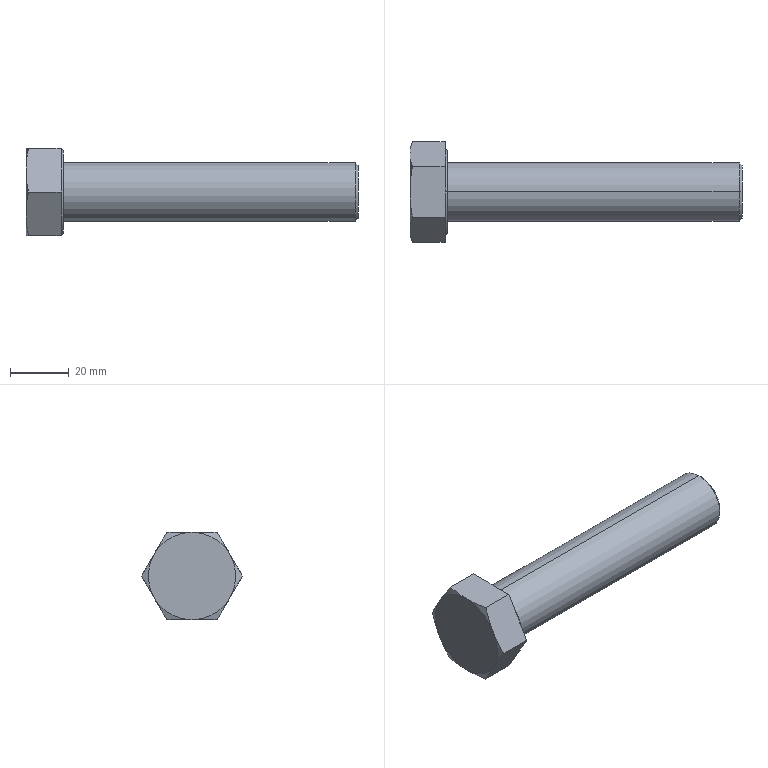Part | 1 solid | 27 faces | box 112.715 x 34.26 x 29.67 mm | volume 40979 mm3 | plane 15 | cone 10 | cylinder 2 | commonest cylinder face diameters 20 x2
STEP:
#1=CARTESIAN_POINT('',(112.715,0.,-9.));
#2=VERTEX_POINT('',#1);
#3=CARTESIAN_POINT('',(112.715,0.,9.));
#4=VERTEX_POINT('',#3);
#5=CARTESIAN_POINT('',(112.715,0.,0.));
#6=DIRECTION('',(1.,0.,0.));
#7=DIRECTION('',(0.,0.,-1.));
#8=AXIS2_PLACEMENT_3D('',#5,#6,#7);
#9=CIRCLE('',#8,9.);
#10=EDGE_CURVE('',#2,#4,#9,.T.);
#11=ORIENTED_EDGE('',*,*,#10,.F.);
#12=CARTESIAN_POINT('',(111.715,0.,-10.));
#13=VERTEX_POINT('',#12);
#14=CARTESIAN_POINT('',(112.715,0.,-9.));
#15=DIRECTION('',(-0.7071,0.,-0.7071));
#16=VECTOR('',#15,1000.);
#17=LINE('',#14,#16);
#18=EDGE_CURVE('',#2,#13,#17,.T.);
#19=ORIENTED_EDGE('',*,*,#18,.T.);
#20=CARTESIAN_POINT('',(111.715,0.,10.));
#21=VERTEX_POINT('',#20);
#22=CARTESIAN_POINT('',(111.715,0.,0.));
#23=DIRECTION('',(-1.,0.,0.));
#24=DIRECTION('',(0.,0.,-1.));
#25=AXIS2_PLACEMENT_3D('',#22,#23,#24);
#26=CIRCLE('',#25,10.);
#27=EDGE_CURVE('',#21,#13,#26,.T.);
#28=ORIENTED_EDGE('',*,*,#27,.F.);
#29=CARTESIAN_POINT('',(112.715,0.,9.));
#30=DIRECTION('',(-0.7071,0.,0.7071));
#31=VECTOR('',#30,1000.);
#32=LINE('',#29,#31);
#33=EDGE_CURVE('',#4,#21,#32,.T.);
#34=ORIENTED_EDGE('',*,*,#33,.F.);
#35=EDGE_LOOP('',(#11,#19,#28,#34));
#36=FACE_OUTER_BOUND('',#35,.T.);
#37=CARTESIAN_POINT('',(112.715,0.,0.));
#38=DIRECTION('',(-1.,0.,0.));
#39=DIRECTION('',(0.,0.,1.));
#40=AXIS2_PLACEMENT_3D('',#37,#38,#39);
#41=CONICAL_SURFACE('',#40,9.,0.7854);
#42=ADVANCED_FACE('',(#36),#41,.T.);
#43=ORIENTED_EDGE('',*,*,#27,.T.);
#44=CARTESIAN_POINT('',(12.715,0.,-10.));
#45=VERTEX_POINT('',#44);
#46=CARTESIAN_POINT('',(112.715,0.,-10.));
#47=DIRECTION('',(-1.,0.,0.));
#48=VECTOR('',#47,1000.);
#49=LINE('',#46,#48);
#50=EDGE_CURVE('',#13,#45,#49,.T.);
#51=ORIENTED_EDGE('',*,*,#50,.T.);
#52=CARTESIAN_POINT('',(12.715,0.,10.));
#53=VERTEX_POINT('',#52);
#54=CARTESIAN_POINT('',(12.715,0.,0.));
#55=DIRECTION('',(1.,0.,0.));
#56=DIRECTION('',(0.,0.,-1.));
#57=AXIS2_PLACEMENT_3D('',#54,#55,#56);
#58=CIRCLE('',#57,10.);
#59=EDGE_CURVE('',#45,#53,#58,.T.);
#60=ORIENTED_EDGE('',*,*,#59,.T.);
#61=CARTESIAN_POINT('',(112.715,0.,10.));
#62=DIRECTION('',(-1.,0.,0.));
#63=VECTOR('',#62,1000.);
#64=LINE('',#61,#63);
#65=EDGE_CURVE('',#21,#53,#64,.T.);
#66=ORIENTED_EDGE('',*,*,#65,.F.);
#67=EDGE_LOOP('',(#43,#51,#60,#66));
#68=FACE_OUTER_BOUND('',#67,.T.);
#69=CARTESIAN_POINT('',(112.715,0.,0.));
#70=DIRECTION('',(-1.,0.,0.));
#71=DIRECTION('',(0.,0.,1.));
#72=AXIS2_PLACEMENT_3D('',#69,#70,#71);
#73=CYLINDRICAL_SURFACE('',#72,10.);
#74=ADVANCED_FACE('',(#68),#73,.T.);
#75=CARTESIAN_POINT('',(12.715,0.,14.095));
#76=VERTEX_POINT('',#75);
#77=CARTESIAN_POINT('',(12.715,0.,-14.095));
#78=VERTEX_POINT('',#77);
#79=CARTESIAN_POINT('',(12.715,0.,0.));
#80=DIRECTION('',(-1.,0.,0.));
#81=DIRECTION('',(0.,0.,1.));
#82=AXIS2_PLACEMENT_3D('',#79,#80,#81);
#83=CIRCLE('',#82,14.095);
#84=EDGE_CURVE('',#76,#78,#83,.T.);
#85=ORIENTED_EDGE('',*,*,#84,.T.);
#86=CARTESIAN_POINT('',(11.975,0.,-14.835));
#87=VERTEX_POINT('',#86);
#88=CARTESIAN_POINT('',(11.915,0.,-14.895));
#89=DIRECTION('',(-0.7071,0.,-0.7071));
#90=VECTOR('',#89,1000.);
#91=LINE('',#88,#90);
#92=EDGE_CURVE('',#78,#87,#91,.T.);
#93=ORIENTED_EDGE('',*,*,#92,.T.);
#94=CARTESIAN_POINT('',(11.915,1.336,-14.835));
#95=VERTEX_POINT('',#94);
#96=CARTESIAN_POINT('',(11.975,0.,-14.835));
#97=CARTESIAN_POINT('',(11.975,0.4454,-14.835));
#98=CARTESIAN_POINT('',(11.955,0.8906,-14.835));
#99=CARTESIAN_POINT('',(11.915,1.336,-14.835));
#100=B_SPLINE_CURVE_WITH_KNOTS('',3,(#96,#97,#98,#99),.UNSPECIFIED.,.F.,.F.,(4,4),(0.008338,0.009669),.UNSPECIFIED.);
#101=EDGE_CURVE('',#87,#95,#100,.T.);
#102=ORIENTED_EDGE('',*,*,#101,.T.);
#103=CARTESIAN_POINT('',(11.915,12.18,-8.574));
#104=VERTEX_POINT('',#103);
#105=CARTESIAN_POINT('',(11.915,0.,0.));
#106=DIRECTION('',(-1.,0.,0.));
#107=DIRECTION('',(0.,0.,1.));
#108=AXIS2_PLACEMENT_3D('',#105,#106,#107);
#109=CIRCLE('',#108,14.895);
#110=EDGE_CURVE('',#104,#95,#109,.T.);
#111=ORIENTED_EDGE('',*,*,#110,.F.);
#112=CARTESIAN_POINT('',(11.915,13.515,-6.261));
#113=VERTEX_POINT('',#112);
#114=CARTESIAN_POINT('',(11.915,12.18,-8.574));
#115=CARTESIAN_POINT('',(11.995,12.625,-7.803));
#116=CARTESIAN_POINT('',(11.995,13.07,-7.032));
#117=CARTESIAN_POINT('',(11.915,13.515,-6.261));
#118=B_SPLINE_CURVE_WITH_KNOTS('',3,(#114,#115,#116,#117),.UNSPECIFIED.,.F.,.F.,(4,4),(0.000002229,0.002673),.UNSPECIFIED.);
#119=EDGE_CURVE('',#104,#113,#118,.T.);
#120=ORIENTED_EDGE('',*,*,#119,.T.);
#121=CARTESIAN_POINT('',(11.915,13.515,6.261));
#122=VERTEX_POINT('',#121);
#123=CARTESIAN_POINT('',(11.915,0.,0.));
#124=DIRECTION('',(-1.,0.,0.));
#125=DIRECTION('',(0.,0.,1.));
#126=AXIS2_PLACEMENT_3D('',#123,#124,#125);
#127=CIRCLE('',#126,14.895);
#128=EDGE_CURVE('',#122,#113,#127,.T.);
#129=ORIENTED_EDGE('',*,*,#128,.F.);
#130=CARTESIAN_POINT('',(11.915,12.18,8.574));
#131=VERTEX_POINT('',#130);
#132=CARTESIAN_POINT('',(11.915,13.515,6.261));
#133=CARTESIAN_POINT('',(11.995,13.07,7.032));
#134=CARTESIAN_POINT('',(11.995,12.625,7.803));
#135=CARTESIAN_POINT('',(11.915,12.18,8.574));
#136=B_SPLINE_CURVE_WITH_KNOTS('',3,(#132,#133,#134,#135),.UNSPECIFIED.,.F.,.F.,(4,4),(0.000002229,0.002673),.UNSPECIFIED.);
#137=EDGE_CURVE('',#122,#131,#136,.T.);
#138=ORIENTED_EDGE('',*,*,#137,.T.);
#139=CARTESIAN_POINT('',(11.915,1.336,14.835));
#140=VERTEX_POINT('',#139);
#141=CARTESIAN_POINT('',(11.915,0.,0.));
#142=DIRECTION('',(-1.,0.,0.));
#143=DIRECTION('',(0.,0.,1.));
#144=AXIS2_PLACEMENT_3D('',#141,#142,#143);
#145=CIRCLE('',#144,14.895);
#146=EDGE_CURVE('',#140,#131,#145,.T.);
#147=ORIENTED_EDGE('',*,*,#146,.F.);
#148=CARTESIAN_POINT('',(11.975,0.,14.835));
#149=VERTEX_POINT('',#148);
#150=CARTESIAN_POINT('',(11.915,1.336,14.835));
#151=CARTESIAN_POINT('',(11.955,0.8906,14.835));
#152=CARTESIAN_POINT('',(11.975,0.4454,14.835));
#153=CARTESIAN_POINT('',(11.975,0.,14.835));
#154=B_SPLINE_CURVE_WITH_KNOTS('',3,(#150,#151,#152,#153),.UNSPECIFIED.,.F.,.F.,(4,4),(0.007682,0.009012),.UNSPECIFIED.);
#155=EDGE_CURVE('',#140,#149,#154,.T.);
#156=ORIENTED_EDGE('',*,*,#155,.T.);
#157=CARTESIAN_POINT('',(11.915,0.,14.895));
#158=DIRECTION('',(-0.7071,0.,0.7071));
#159=VECTOR('',#158,1000.);
#160=LINE('',#157,#159);
#161=EDGE_CURVE('',#76,#149,#160,.T.);
#162=ORIENTED_EDGE('',*,*,#161,.F.);
#163=EDGE_LOOP('',(#85,#93,#102,#111,#120,#129,#138,#147,#156,#162));
#164=FACE_OUTER_BOUND('',#163,.T.);
#165=CARTESIAN_POINT('',(11.915,0.,0.));
#166=DIRECTION('',(-1.,0.,0.));
#167=DIRECTION('',(0.,0.,1.));
#168=AXIS2_PLACEMENT_3D('',#165,#166,#167);
#169=CONICAL_SURFACE('',#168,14.895,0.7854);
#170=ADVANCED_FACE('',(#164),#169,.T.);
#171=ORIENTED_EDGE('',*,*,#84,.F.);
#172=CARTESIAN_POINT('',(12.715,0.,0.));
#173=DIRECTION('',(-1.,0.,0.));
#174=DIRECTION('',(0.,0.,1.));
#175=AXIS2_PLACEMENT_3D('',#172,#173,#174);
#176=CIRCLE('',#175,14.095);
#177=EDGE_CURVE('',#78,#76,#176,.T.);
#178=ORIENTED_EDGE('',*,*,#177,.F.);
#179=EDGE_LOOP('',(#171,#178));
#180=FACE_OUTER_BOUND('',#179,.T.);
#181=CARTESIAN_POINT('',(12.715,0.,0.));
#182=DIRECTION('',(1.,0.,0.));
#183=DIRECTION('',(0.,0.,-1.));
#184=AXIS2_PLACEMENT_3D('',#181,#182,#183);
#185=CIRCLE('',#184,10.);
#186=EDGE_CURVE('',#53,#45,#185,.T.);
#187=ORIENTED_EDGE('',*,*,#186,.F.);
#188=ORIENTED_EDGE('',*,*,#59,.F.);
#189=EDGE_LOOP('',(#187,#188));
#190=FACE_BOUND('',#189,.T.);
#191=CARTESIAN_POINT('',(12.715,-8.565,-14.835));
#192=DIRECTION('',(1.,0.,0.));
#193=DIRECTION('',(0.,0.,-1.));
#194=AXIS2_PLACEMENT_3D('',#191,#192,#193);
#195=PLANE('',#194);
#196=ADVANCED_FACE('',(#180,#190),#195,.T.);
#197=CARTESIAN_POINT('',(0.8353,-8.565,-14.835));
#198=VERTEX_POINT('',#197);
#199=CARTESIAN_POINT('',(0.,-12.847,-7.417));
#200=VERTEX_POINT('',#199);
#201=CARTESIAN_POINT('',(0.8353,-8.565,-14.835));
#202=CARTESIAN_POINT('',(0.5755,-9.279,-13.599));
#203=CARTESIAN_POINT('',(0.3646,-9.992,-12.362));
#204=CARTESIAN_POINT('',(0.07638,-11.42,-9.89));
#205=CARTESIAN_POINT('',(0.,-12.134,-8.654));
#206=CARTESIAN_POINT('',(0.,-12.847,-7.417));
#207=B_SPLINE_CURVE_WITH_KNOTS('',3,(#201,#202,#203,#204,#205,#206),.UNSPECIFIED.,.F.,.F.,(4,2,4),(0.000000231,0.004283,0.008565),.UNSPECIFIED.);
#208=EDGE_CURVE('',#198,#200,#207,.T.);
#209=ORIENTED_EDGE('',*,*,#208,.F.);
#210=CARTESIAN_POINT('',(11.915,-8.565,-14.835));
#211=VERTEX_POINT('',#210);
#212=CARTESIAN_POINT('',(12.715,-8.565,-14.835));
#213=DIRECTION('',(-1.,0.,0.));
#214=VECTOR('',#213,1000.);
#215=LINE('',#212,#214);
#216=EDGE_CURVE('',#211,#198,#215,.T.);
#217=ORIENTED_EDGE('',*,*,#216,.F.);
#218=CARTESIAN_POINT('',(11.915,-12.18,-8.574));
#219=VERTEX_POINT('',#218);
#220=CARTESIAN_POINT('',(11.915,-17.13,0.));
#221=DIRECTION('',(0.,0.5,-0.866));
#222=VECTOR('',#221,1000.);
#223=LINE('',#220,#222);
#224=EDGE_CURVE('',#219,#211,#223,.T.);
#225=ORIENTED_EDGE('',*,*,#224,.F.);
#226=CARTESIAN_POINT('',(11.915,-13.515,-6.261));
#227=VERTEX_POINT('',#226);
#228=CARTESIAN_POINT('',(11.915,-13.515,-6.261));
#229=CARTESIAN_POINT('',(11.995,-13.07,-7.032));
#230=CARTESIAN_POINT('',(11.995,-12.625,-7.803));
#231=CARTESIAN_POINT('',(11.915,-12.18,-8.574));
#232=B_SPLINE_CURVE_WITH_KNOTS('',3,(#228,#229,#230,#231),.UNSPECIFIED.,.F.,.F.,(4,4),(0.000002229,0.002673),.UNSPECIFIED.);
#233=EDGE_CURVE('',#227,#219,#232,.T.);
#234=ORIENTED_EDGE('',*,*,#233,.F.);
#235=CARTESIAN_POINT('',(11.915,-17.13,0.));
#236=VERTEX_POINT('',#235);
#237=CARTESIAN_POINT('',(11.915,-17.13,0.));
#238=DIRECTION('',(0.,0.5,-0.866));
#239=VECTOR('',#238,1000.);
#240=LINE('',#237,#239);
#241=EDGE_CURVE('',#236,#227,#240,.T.);
#242=ORIENTED_EDGE('',*,*,#241,.F.);
#243=CARTESIAN_POINT('',(0.8353,-17.13,0.));
#244=VERTEX_POINT('',#243);
#245=CARTESIAN_POINT('',(12.715,-17.13,0.));
#246=DIRECTION('',(-1.,0.,0.));
#247=VECTOR('',#246,1000.);
#248=LINE('',#245,#247);
#249=EDGE_CURVE('',#236,#244,#248,.T.);
#250=ORIENTED_EDGE('',*,*,#249,.T.);
#251=CARTESIAN_POINT('',(0.,-12.847,-7.417));
#252=CARTESIAN_POINT('',(0.,-13.561,-6.181));
#253=CARTESIAN_POINT('',(0.07638,-14.275,-4.945));
#254=CARTESIAN_POINT('',(0.3646,-15.702,-2.473));
#255=CARTESIAN_POINT('',(0.5755,-16.416,-1.236));
#256=CARTESIAN_POINT('',(0.8353,-17.13,0.));
#257=B_SPLINE_CURVE_WITH_KNOTS('',3,(#251,#252,#253,#254,#255,#256),.UNSPECIFIED.,.F.,.F.,(4,2,4),(0.008565,0.01285,0.01713),.UNSPECIFIED.);
#258=EDGE_CURVE('',#200,#244,#257,.T.);
#259=ORIENTED_EDGE('',*,*,#258,.F.);
#260=EDGE_LOOP('',(#209,#217,#225,#234,#242,#250,#259));
#261=FACE_OUTER_BOUND('',#260,.T.);
#262=CARTESIAN_POINT('',(12.715,-17.13,0.));
#263=DIRECTION('',(0.,0.866,0.5));
#264=DIRECTION('',(0.,-0.5,0.866));
#265=AXIS2_PLACEMENT_3D('',#262,#263,#264);
#266=PLANE('',#265);
#267=ADVANCED_FACE('',(#261),#266,.F.);
#268=CARTESIAN_POINT('',(0.8353,8.565,-14.835));
#269=VERTEX_POINT('',#268);
#270=CARTESIAN_POINT('',(0.,0.,-14.835));
#271=VERTEX_POINT('',#270);
#272=CARTESIAN_POINT('',(0.8353,8.565,-14.835));
#273=CARTESIAN_POINT('',(0.5762,7.141,-14.835));
#274=CARTESIAN_POINT('',(0.3651,5.714,-14.835));
#275=CARTESIAN_POINT('',(0.07668,2.859,-14.835));
#276=CARTESIAN_POINT('',(0.,1.43,-14.835));
#277=CARTESIAN_POINT('',(0.,0.,-14.835));
#278=B_SPLINE_CURVE_WITH_KNOTS('',3,(#272,#273,#274,#275,#276,#277),.UNSPECIFIED.,.F.,.F.,(4,2,4),(0.03088,0.0352,0.03952),.UNSPECIFIED.);
#279=EDGE_CURVE('',#269,#271,#278,.T.);
#280=ORIENTED_EDGE('',*,*,#279,.F.);
#281=CARTESIAN_POINT('',(11.915,8.565,-14.835));
#282=VERTEX_POINT('',#281);
#283=CARTESIAN_POINT('',(12.715,8.565,-14.835));
#284=DIRECTION('',(-1.,0.,0.));
#285=VECTOR('',#284,1000.);
#286=LINE('',#283,#285);
#287=EDGE_CURVE('',#282,#269,#286,.T.);
#288=ORIENTED_EDGE('',*,*,#287,.F.);
#289=CARTESIAN_POINT('',(11.915,-8.565,-14.835));
#290=DIRECTION('',(0.,1.,0.));
#291=VECTOR('',#290,1000.);
#292=LINE('',#289,#291);
#293=EDGE_CURVE('',#95,#282,#292,.T.);
#294=ORIENTED_EDGE('',*,*,#293,.F.);
#295=ORIENTED_EDGE('',*,*,#101,.F.);
#296=CARTESIAN_POINT('',(11.915,-1.336,-14.835));
#297=VERTEX_POINT('',#296);
#298=CARTESIAN_POINT('',(11.915,-1.336,-14.835));
#299=CARTESIAN_POINT('',(11.955,-0.8902,-14.835));
#300=CARTESIAN_POINT('',(11.975,-0.445,-14.835));
#301=CARTESIAN_POINT('',(11.975,0.,-14.835));
#302=B_SPLINE_CURVE_WITH_KNOTS('',3,(#298,#299,#300,#301),.UNSPECIFIED.,.F.,.F.,(4,4),(0.007008,0.008338),.UNSPECIFIED.);
#303=EDGE_CURVE('',#297,#87,#302,.T.);
#304=ORIENTED_EDGE('',*,*,#303,.F.);
#305=CARTESIAN_POINT('',(11.915,-8.565,-14.835));
#306=DIRECTION('',(0.,1.,0.));
#307=VECTOR('',#306,1000.);
#308=LINE('',#305,#307);
#309=EDGE_CURVE('',#211,#297,#308,.T.);
#310=ORIENTED_EDGE('',*,*,#309,.F.);
#311=ORIENTED_EDGE('',*,*,#216,.T.);
#312=CARTESIAN_POINT('',(0.,0.,-14.835));
#313=CARTESIAN_POINT('',(0.,-1.426,-14.835));
#314=CARTESIAN_POINT('',(0.07627,-2.854,-14.835));
#315=CARTESIAN_POINT('',(0.3649,-5.713,-14.835));
#316=CARTESIAN_POINT('',(0.5772,-7.147,-14.835));
#317=CARTESIAN_POINT('',(0.8353,-8.565,-14.835));
#318=B_SPLINE_CURVE_WITH_KNOTS('',3,(#312,#313,#314,#315,#316,#317),.UNSPECIFIED.,.F.,.F.,(4,2,4),(0.03952,0.04383,0.04813),.UNSPECIFIED.);
#319=EDGE_CURVE('',#271,#198,#318,.T.);
#320=ORIENTED_EDGE('',*,*,#319,.F.);
#321=EDGE_LOOP('',(#280,#288,#294,#295,#304,#310,#311,#320));
#322=FACE_OUTER_BOUND('',#321,.T.);
#323=CARTESIAN_POINT('',(12.715,-8.565,-14.835));
#324=DIRECTION('',(0.,0.,1.));
#325=DIRECTION('',(1.,0.,0.));
#326=AXIS2_PLACEMENT_3D('',#323,#324,#325);
#327=PLANE('',#326);
#328=ADVANCED_FACE('',(#322),#327,.F.);
#329=CARTESIAN_POINT('',(0.8353,17.13,0.));
#330=VERTEX_POINT('',#329);
#331=CARTESIAN_POINT('',(0.,12.847,-7.417));
#332=VERTEX_POINT('',#331);
#333=CARTESIAN_POINT('',(0.8353,17.13,0.));
#334=CARTESIAN_POINT('',(0.5755,16.416,-1.236));
#335=CARTESIAN_POINT('',(0.3646,15.702,-2.473));
#336=CARTESIAN_POINT('',(0.07638,14.275,-4.945));
#337=CARTESIAN_POINT('',(0.,13.561,-6.181));
#338=CARTESIAN_POINT('',(0.,12.847,-7.417));
#339=B_SPLINE_CURVE_WITH_KNOTS('',3,(#333,#334,#335,#336,#337,#338),.UNSPECIFIED.,.F.,.F.,(4,2,4),(0.000000231,0.004283,0.008565),.UNSPECIFIED.);
#340=EDGE_CURVE('',#330,#332,#339,.T.);
#341=ORIENTED_EDGE('',*,*,#340,.F.);
#342=CARTESIAN_POINT('',(11.915,17.13,0.));
#343=VERTEX_POINT('',#342);
#344=CARTESIAN_POINT('',(12.715,17.13,0.));
#345=DIRECTION('',(-1.,0.,0.));
#346=VECTOR('',#345,1000.);
#347=LINE('',#344,#346);
#348=EDGE_CURVE('',#343,#330,#347,.T.);
#349=ORIENTED_EDGE('',*,*,#348,.F.);
#350=CARTESIAN_POINT('',(11.915,8.565,-14.835));
#351=DIRECTION('',(0.,0.5,0.866));
#352=VECTOR('',#351,1000.);
#353=LINE('',#350,#352);
#354=EDGE_CURVE('',#113,#343,#353,.T.);
#355=ORIENTED_EDGE('',*,*,#354,.F.);
#356=ORIENTED_EDGE('',*,*,#119,.F.);
#357=CARTESIAN_POINT('',(11.915,8.565,-14.835));
#358=DIRECTION('',(0.,0.5,0.866));
#359=VECTOR('',#358,1000.);
#360=LINE('',#357,#359);
#361=EDGE_CURVE('',#282,#104,#360,.T.);
#362=ORIENTED_EDGE('',*,*,#361,.F.);
#363=ORIENTED_EDGE('',*,*,#287,.T.);
#364=CARTESIAN_POINT('',(0.,12.847,-7.417));
#365=CARTESIAN_POINT('',(0.,12.134,-8.654));
#366=CARTESIAN_POINT('',(0.07638,11.42,-9.89));
#367=CARTESIAN_POINT('',(0.3646,9.992,-12.363));
#368=CARTESIAN_POINT('',(0.5755,9.279,-13.599));
#369=CARTESIAN_POINT('',(0.8353,8.565,-14.835));
#370=B_SPLINE_CURVE_WITH_KNOTS('',3,(#364,#365,#366,#367,#368,#369),.UNSPECIFIED.,.F.,.F.,(4,2,4),(0.008565,0.01285,0.01713),.UNSPECIFIED.);
#371=EDGE_CURVE('',#332,#269,#370,.T.);
#372=ORIENTED_EDGE('',*,*,#371,.F.);
#373=EDGE_LOOP('',(#341,#349,#355,#356,#362,#363,#372));
#374=FACE_OUTER_BOUND('',#373,.T.);
#375=CARTESIAN_POINT('',(12.715,8.565,-14.835));
#376=DIRECTION('',(0.,-0.866,0.5));
#377=DIRECTION('',(0.,-0.5,-0.866));
#378=AXIS2_PLACEMENT_3D('',#375,#376,#377);
#379=PLANE('',#378);
#380=ADVANCED_FACE('',(#374),#379,.F.);
#381=CARTESIAN_POINT('',(0.8353,8.565,14.835));
#382=VERTEX_POINT('',#381);
#383=CARTESIAN_POINT('',(0.,12.847,7.417));
#384=VERTEX_POINT('',#383);
#385=CARTESIAN_POINT('',(0.8353,8.565,14.835));
#386=CARTESIAN_POINT('',(0.5755,9.279,13.599));
#387=CARTESIAN_POINT('',(0.3646,9.992,12.363));
#388=CARTESIAN_POINT('',(0.07638,11.42,9.89));
#389=CARTESIAN_POINT('',(0.,12.134,8.654));
#390=CARTESIAN_POINT('',(0.,12.847,7.417));
#391=B_SPLINE_CURVE_WITH_KNOTS('',3,(#385,#386,#387,#388,#389,#390),.UNSPECIFIED.,.F.,.F.,(4,2,4),(0.000000231,0.004283,0.008565),.UNSPECIFIED.);
#392=EDGE_CURVE('',#382,#384,#391,.T.);
#393=ORIENTED_EDGE('',*,*,#392,.F.);
#394=CARTESIAN_POINT('',(11.915,8.565,14.835));
#395=VERTEX_POINT('',#394);
#396=CARTESIAN_POINT('',(12.715,8.565,14.835));
#397=DIRECTION('',(-1.,0.,0.));
#398=VECTOR('',#397,1000.);
#399=LINE('',#396,#398);
#400=EDGE_CURVE('',#395,#382,#399,.T.);
#401=ORIENTED_EDGE('',*,*,#400,.F.);
#402=CARTESIAN_POINT('',(11.915,17.13,0.));
#403=DIRECTION('',(0.,-0.5,0.866));
#404=VECTOR('',#403,1000.);
#405=LINE('',#402,#404);
#406=EDGE_CURVE('',#131,#395,#405,.T.);
#407=ORIENTED_EDGE('',*,*,#406,.F.);
#408=ORIENTED_EDGE('',*,*,#137,.F.);
#409=CARTESIAN_POINT('',(11.915,17.13,0.));
#410=DIRECTION('',(0.,-0.5,0.866));
#411=VECTOR('',#410,1000.);
#412=LINE('',#409,#411);
#413=EDGE_CURVE('',#343,#122,#412,.T.);
#414=ORIENTED_EDGE('',*,*,#413,.F.);
#415=ORIENTED_EDGE('',*,*,#348,.T.);
#416=CARTESIAN_POINT('',(0.,12.847,7.417));
#417=CARTESIAN_POINT('',(0.,13.561,6.181));
#418=CARTESIAN_POINT('',(0.07638,14.275,4.945));
#419=CARTESIAN_POINT('',(0.3646,15.702,2.473));
#420=CARTESIAN_POINT('',(0.5755,16.416,1.236));
#421=CARTESIAN_POINT('',(0.8353,17.13,0.));
#422=B_SPLINE_CURVE_WITH_KNOTS('',3,(#416,#417,#418,#419,#420,#421),.UNSPECIFIED.,.F.,.F.,(4,2,4),(0.008565,0.01285,0.01713),.UNSPECIFIED.);
#423=EDGE_CURVE('',#384,#330,#422,.T.);
#424=ORIENTED_EDGE('',*,*,#423,.F.);
#425=EDGE_LOOP('',(#393,#401,#407,#408,#414,#415,#424));
#426=FACE_OUTER_BOUND('',#425,.T.);
#427=CARTESIAN_POINT('',(12.715,17.13,0.));
#428=DIRECTION('',(0.,-0.866,-0.5));
#429=DIRECTION('',(0.,0.5,-0.866));
#430=AXIS2_PLACEMENT_3D('',#427,#428,#429);
#431=PLANE('',#430);
#432=ADVANCED_FACE('',(#426),#431,.F.);
#433=CARTESIAN_POINT('',(0.8353,-8.565,14.835));
#434=VERTEX_POINT('',#433);
#435=CARTESIAN_POINT('',(0.,0.,14.835));
#436=VERTEX_POINT('',#435);
#437=CARTESIAN_POINT('',(0.8353,-8.565,14.835));
#438=CARTESIAN_POINT('',(0.5772,-7.147,14.835));
#439=CARTESIAN_POINT('',(0.3649,-5.713,14.835));
#440=CARTESIAN_POINT('',(0.07627,-2.854,14.835));
#441=CARTESIAN_POINT('',(0.,-1.426,14.835));
#442=CARTESIAN_POINT('',(0.,0.,14.835));
#443=B_SPLINE_CURVE_WITH_KNOTS('',3,(#437,#438,#439,#440,#441,#442),.UNSPECIFIED.,.F.,.F.,(4,2,4),(0.01457,0.01889,0.0232),.UNSPECIFIED.);
#444=EDGE_CURVE('',#434,#436,#443,.T.);
#445=ORIENTED_EDGE('',*,*,#444,.F.);
#446=CARTESIAN_POINT('',(11.915,-8.565,14.835));
#447=VERTEX_POINT('',#446);
#448=CARTESIAN_POINT('',(12.715,-8.565,14.835));
#449=DIRECTION('',(-1.,0.,0.));
#450=VECTOR('',#449,1000.);
#451=LINE('',#448,#450);
#452=EDGE_CURVE('',#447,#434,#451,.T.);
#453=ORIENTED_EDGE('',*,*,#452,.F.);
#454=CARTESIAN_POINT('',(11.915,-1.336,14.835));
#455=VERTEX_POINT('',#454);
#456=CARTESIAN_POINT('',(11.915,8.565,14.835));
#457=DIRECTION('',(0.,-1.,0.));
#458=VECTOR('',#457,1000.);
#459=LINE('',#456,#458);
#460=EDGE_CURVE('',#455,#447,#459,.T.);
#461=ORIENTED_EDGE('',*,*,#460,.F.);
#462=CARTESIAN_POINT('',(11.975,0.,14.835));
#463=CARTESIAN_POINT('',(11.975,-0.445,14.835));
#464=CARTESIAN_POINT('',(11.955,-0.8902,14.835));
#465=CARTESIAN_POINT('',(11.915,-1.336,14.835));
#466=B_SPLINE_CURVE_WITH_KNOTS('',3,(#462,#463,#464,#465),.UNSPECIFIED.,.F.,.F.,(4,4),(0.009012,0.01034),.UNSPECIFIED.);
#467=EDGE_CURVE('',#149,#455,#466,.T.);
#468=ORIENTED_EDGE('',*,*,#467,.F.);
#469=ORIENTED_EDGE('',*,*,#155,.F.);
#470=CARTESIAN_POINT('',(11.915,8.565,14.835));
#471=DIRECTION('',(0.,-1.,0.));
#472=VECTOR('',#471,1000.);
#473=LINE('',#470,#472);
#474=EDGE_CURVE('',#395,#140,#473,.T.);
#475=ORIENTED_EDGE('',*,*,#474,.F.);
#476=ORIENTED_EDGE('',*,*,#400,.T.);
#477=CARTESIAN_POINT('',(0.,0.,14.835));
#478=CARTESIAN_POINT('',(0.,1.43,14.835));
#479=CARTESIAN_POINT('',(0.07668,2.859,14.835));
#480=CARTESIAN_POINT('',(0.3651,5.714,14.835));
#481=CARTESIAN_POINT('',(0.5762,7.141,14.835));
#482=CARTESIAN_POINT('',(0.8353,8.565,14.835));
#483=B_SPLINE_CURVE_WITH_KNOTS('',3,(#477,#478,#479,#480,#481,#482),.UNSPECIFIED.,.F.,.F.,(4,2,4),(0.0232,0.02753,0.03186),.UNSPECIFIED.);
#484=EDGE_CURVE('',#436,#382,#483,.T.);
#485=ORIENTED_EDGE('',*,*,#484,.F.);
#486=EDGE_LOOP('',(#445,#453,#461,#468,#469,#475,#476,#485));
#487=FACE_OUTER_BOUND('',#486,.T.);
#488=CARTESIAN_POINT('',(12.715,8.565,14.835));
#489=DIRECTION('',(0.,0.,-1.));
#490=DIRECTION('',(-1.,0.,0.));
#491=AXIS2_PLACEMENT_3D('',#488,#489,#490);
#492=PLANE('',#491);
#493=ADVANCED_FACE('',(#487),#492,.F.);
#494=CARTESIAN_POINT('',(0.,-12.847,7.417));
#495=VERTEX_POINT('',#494);
#496=CARTESIAN_POINT('',(0.8353,-17.13,0.));
#497=CARTESIAN_POINT('',(0.5755,-16.416,1.236));
#498=CARTESIAN_POINT('',(0.3646,-15.702,2.472));
#499=CARTESIAN_POINT('',(0.07638,-14.275,4.945));
#500=CARTESIAN_POINT('',(0.,-13.561,6.181));
#501=CARTESIAN_POINT('',(0.,-12.847,7.417));
#502=B_SPLINE_CURVE_WITH_KNOTS('',3,(#496,#497,#498,#499,#500,#501),.UNSPECIFIED.,.F.,.F.,(4,2,4),(0.000000231,0.004283,0.008565),.UNSPECIFIED.);
#503=EDGE_CURVE('',#244,#495,#502,.T.);
#504=ORIENTED_EDGE('',*,*,#503,.F.);
#505=ORIENTED_EDGE('',*,*,#249,.F.);
#506=CARTESIAN_POINT('',(11.915,-13.515,6.261));
#507=VERTEX_POINT('',#506);
#508=CARTESIAN_POINT('',(11.915,-8.565,14.835));
#509=DIRECTION('',(0.,-0.5,-0.866));
#510=VECTOR('',#509,1000.);
#511=LINE('',#508,#510);
#512=EDGE_CURVE('',#507,#236,#511,.T.);
#513=ORIENTED_EDGE('',*,*,#512,.F.);
#514=CARTESIAN_POINT('',(11.915,-12.18,8.574));
#515=VERTEX_POINT('',#514);
#516=CARTESIAN_POINT('',(11.915,-12.18,8.574));
#517=CARTESIAN_POINT('',(11.995,-12.625,7.803));
#518=CARTESIAN_POINT('',(11.995,-13.07,7.032));
#519=CARTESIAN_POINT('',(11.915,-13.515,6.261));
#520=B_SPLINE_CURVE_WITH_KNOTS('',3,(#516,#517,#518,#519),.UNSPECIFIED.,.F.,.F.,(4,4),(0.000002229,0.002673),.UNSPECIFIED.);
#521=EDGE_CURVE('',#515,#507,#520,.T.);
#522=ORIENTED_EDGE('',*,*,#521,.F.);
#523=CARTESIAN_POINT('',(11.915,-8.565,14.835));
#524=DIRECTION('',(0.,-0.5,-0.866));
#525=VECTOR('',#524,1000.);
#526=LINE('',#523,#525);
#527=EDGE_CURVE('',#447,#515,#526,.T.);
#528=ORIENTED_EDGE('',*,*,#527,.F.);
#529=ORIENTED_EDGE('',*,*,#452,.T.);
#530=CARTESIAN_POINT('',(0.,-12.847,7.417));
#531=CARTESIAN_POINT('',(0.,-12.134,8.654));
#532=CARTESIAN_POINT('',(0.07638,-11.42,9.89));
#533=CARTESIAN_POINT('',(0.3646,-9.992,12.363));
#534=CARTESIAN_POINT('',(0.5755,-9.279,13.599));
#535=CARTESIAN_POINT('',(0.8353,-8.565,14.835));
#536=B_SPLINE_CURVE_WITH_KNOTS('',3,(#530,#531,#532,#533,#534,#535),.UNSPECIFIED.,.F.,.F.,(4,2,4),(0.008565,0.01285,0.01713),.UNSPECIFIED.);
#537=EDGE_CURVE('',#495,#434,#536,.T.);
#538=ORIENTED_EDGE('',*,*,#537,.F.);
#539=EDGE_LOOP('',(#504,#505,#513,#522,#528,#529,#538));
#540=FACE_OUTER_BOUND('',#539,.T.);
#541=CARTESIAN_POINT('',(12.715,-8.565,14.835));
#542=DIRECTION('',(0.,0.866,-0.5));
#543=DIRECTION('',(0.,0.5,0.866));
#544=AXIS2_PLACEMENT_3D('',#541,#542,#543);
#545=PLANE('',#544);
#546=ADVANCED_FACE('',(#540),#545,.F.);
#547=ORIENTED_EDGE('',*,*,#224,.T.);
#548=ORIENTED_EDGE('',*,*,#309,.T.);
#549=CARTESIAN_POINT('',(11.915,0.,0.));
#550=DIRECTION('',(-1.,0.,0.));
#551=DIRECTION('',(0.,0.,1.));
#552=AXIS2_PLACEMENT_3D('',#549,#550,#551);
#553=CIRCLE('',#552,14.895);
#554=EDGE_CURVE('',#297,#219,#553,.T.);
#555=ORIENTED_EDGE('',*,*,#554,.T.);
#556=EDGE_LOOP('',(#547,#548,#555));
#557=FACE_OUTER_BOUND('',#556,.T.);
#558=CARTESIAN_POINT('',(11.915,14.895,0.));
#559=DIRECTION('',(1.,0.,0.));
#560=DIRECTION('',(0.,0.,-1.));
#561=AXIS2_PLACEMENT_3D('',#558,#559,#560);
#562=PLANE('',#561);
#563=ADVANCED_FACE('',(#557),#562,.T.);
#564=ORIENTED_EDGE('',*,*,#293,.T.);
#565=ORIENTED_EDGE('',*,*,#361,.T.);
#566=ORIENTED_EDGE('',*,*,#110,.T.);
#567=EDGE_LOOP('',(#564,#565,#566));
#568=FACE_OUTER_BOUND('',#567,.T.);
#569=CARTESIAN_POINT('',(11.915,14.895,0.));
#570=DIRECTION('',(1.,0.,0.));
#571=DIRECTION('',(0.,0.,-1.));
#572=AXIS2_PLACEMENT_3D('',#569,#570,#571);
#573=PLANE('',#572);
#574=ADVANCED_FACE('',(#568),#573,.T.);
#575=ORIENTED_EDGE('',*,*,#354,.T.);
#576=ORIENTED_EDGE('',*,*,#413,.T.);
#577=ORIENTED_EDGE('',*,*,#128,.T.);
#578=EDGE_LOOP('',(#575,#576,#577));
#579=FACE_OUTER_BOUND('',#578,.T.);
#580=CARTESIAN_POINT('',(11.915,14.895,0.));
#581=DIRECTION('',(1.,0.,0.));
#582=DIRECTION('',(0.,0.,-1.));
#583=AXIS2_PLACEMENT_3D('',#580,#581,#582);
#584=PLANE('',#583);
#585=ADVANCED_FACE('',(#579),#584,.T.);
#586=ORIENTED_EDGE('',*,*,#406,.T.);
#587=ORIENTED_EDGE('',*,*,#474,.T.);
#588=ORIENTED_EDGE('',*,*,#146,.T.);
#589=EDGE_LOOP('',(#586,#587,#588));
#590=FACE_OUTER_BOUND('',#589,.T.);
#591=CARTESIAN_POINT('',(11.915,14.895,0.));
#592=DIRECTION('',(1.,0.,0.));
#593=DIRECTION('',(0.,0.,-1.));
#594=AXIS2_PLACEMENT_3D('',#591,#592,#593);
#595=PLANE('',#594);
#596=ADVANCED_FACE('',(#590),#595,.T.);
#597=ORIENTED_EDGE('',*,*,#460,.T.);
#598=ORIENTED_EDGE('',*,*,#527,.T.);
#599=CARTESIAN_POINT('',(11.915,0.,0.));
#600=DIRECTION('',(-1.,0.,0.));
#601=DIRECTION('',(0.,0.,1.));
#602=AXIS2_PLACEMENT_3D('',#599,#600,#601);
#603=CIRCLE('',#602,14.895);
#604=EDGE_CURVE('',#515,#455,#603,.T.);
#605=ORIENTED_EDGE('',*,*,#604,.T.);
#606=EDGE_LOOP('',(#597,#598,#605));
#607=FACE_OUTER_BOUND('',#606,.T.);
#608=CARTESIAN_POINT('',(11.915,14.895,0.));
#609=DIRECTION('',(1.,0.,0.));
#610=DIRECTION('',(0.,0.,-1.));
#611=AXIS2_PLACEMENT_3D('',#608,#609,#610);
#612=PLANE('',#611);
#613=ADVANCED_FACE('',(#607),#612,.T.);
#614=ORIENTED_EDGE('',*,*,#241,.T.);
#615=CARTESIAN_POINT('',(11.915,0.,0.));
#616=DIRECTION('',(-1.,0.,0.));
#617=DIRECTION('',(0.,0.,1.));
#618=AXIS2_PLACEMENT_3D('',#615,#616,#617);
#619=CIRCLE('',#618,14.895);
#620=EDGE_CURVE('',#227,#507,#619,.T.);
#621=ORIENTED_EDGE('',*,*,#620,.T.);
#622=ORIENTED_EDGE('',*,*,#512,.T.);
#623=EDGE_LOOP('',(#614,#621,#622));
#624=FACE_OUTER_BOUND('',#623,.T.);
#625=CARTESIAN_POINT('',(11.915,14.895,0.));
#626=DIRECTION('',(1.,0.,0.));
#627=DIRECTION('',(0.,0.,-1.));
#628=AXIS2_PLACEMENT_3D('',#625,#626,#627);
#629=PLANE('',#628);
#630=ADVANCED_FACE('',(#624),#629,.T.);
#631=ORIENTED_EDGE('',*,*,#92,.F.);
#632=ORIENTED_EDGE('',*,*,#177,.T.);
#633=ORIENTED_EDGE('',*,*,#161,.T.);
#634=ORIENTED_EDGE('',*,*,#467,.T.);
#635=ORIENTED_EDGE('',*,*,#604,.F.);
#636=ORIENTED_EDGE('',*,*,#521,.T.);
#637=ORIENTED_EDGE('',*,*,#620,.F.);
#638=ORIENTED_EDGE('',*,*,#233,.T.);
#639=ORIENTED_EDGE('',*,*,#554,.F.);
#640=ORIENTED_EDGE('',*,*,#303,.T.);
#641=EDGE_LOOP('',(#631,#632,#633,#634,#635,#636,#637,#638,#639,#640));
#642=FACE_OUTER_BOUND('',#641,.T.);
#643=CARTESIAN_POINT('',(11.915,0.,0.));
#644=DIRECTION('',(-1.,0.,0.));
#645=DIRECTION('',(0.,0.,1.));
#646=AXIS2_PLACEMENT_3D('',#643,#644,#645);
#647=CONICAL_SURFACE('',#646,14.895,0.7854);
#648=ADVANCED_FACE('',(#642),#647,.T.);
#649=ORIENTED_EDGE('',*,*,#319,.T.);
#650=ORIENTED_EDGE('',*,*,#208,.T.);
#651=CARTESIAN_POINT('',(0.,0.,0.));
#652=DIRECTION('',(1.,0.,0.));
#653=DIRECTION('',(0.,0.,-1.));
#654=AXIS2_PLACEMENT_3D('',#651,#652,#653);
#655=CIRCLE('',#654,14.835);
#656=EDGE_CURVE('',#200,#271,#655,.T.);
#657=ORIENTED_EDGE('',*,*,#656,.T.);
#658=EDGE_LOOP('',(#649,#650,#657));
#659=FACE_OUTER_BOUND('',#658,.T.);
#660=CARTESIAN_POINT('',(0.,0.,0.));
#661=DIRECTION('',(1.,0.,0.));
#662=DIRECTION('',(0.,0.,-1.));
#663=AXIS2_PLACEMENT_3D('',#660,#661,#662);
#664=CONICAL_SURFACE('',#663,14.835,1.222);
#665=ADVANCED_FACE('',(#659),#664,.T.);
#666=ORIENTED_EDGE('',*,*,#258,.T.);
#667=ORIENTED_EDGE('',*,*,#503,.T.);
#668=CARTESIAN_POINT('',(0.,0.,0.));
#669=DIRECTION('',(1.,0.,0.));
#670=DIRECTION('',(0.,0.,-1.));
#671=AXIS2_PLACEMENT_3D('',#668,#669,#670);
#672=CIRCLE('',#671,14.835);
#673=EDGE_CURVE('',#495,#200,#672,.T.);
#674=ORIENTED_EDGE('',*,*,#673,.T.);
#675=EDGE_LOOP('',(#666,#667,#674));
#676=FACE_OUTER_BOUND('',#675,.T.);
#677=CARTESIAN_POINT('',(0.,0.,0.));
#678=DIRECTION('',(1.,0.,0.));
#679=DIRECTION('',(0.,0.,-1.));
#680=AXIS2_PLACEMENT_3D('',#677,#678,#679);
#681=CONICAL_SURFACE('',#680,14.835,1.222);
#682=ADVANCED_FACE('',(#676),#681,.T.);
#683=ORIENTED_EDGE('',*,*,#444,.T.);
#684=CARTESIAN_POINT('',(0.,0.,0.));
#685=DIRECTION('',(1.,0.,0.));
#686=DIRECTION('',(0.,0.,-1.));
#687=AXIS2_PLACEMENT_3D('',#684,#685,#686);
#688=CIRCLE('',#687,14.835);
#689=EDGE_CURVE('',#436,#495,#688,.T.);
#690=ORIENTED_EDGE('',*,*,#689,.T.);
#691=ORIENTED_EDGE('',*,*,#537,.T.);
#692=EDGE_LOOP('',(#683,#690,#691));
#693=FACE_OUTER_BOUND('',#692,.T.);
#694=CARTESIAN_POINT('',(0.,0.,0.));
#695=DIRECTION('',(1.,0.,0.));
#696=DIRECTION('',(0.,0.,-1.));
#697=AXIS2_PLACEMENT_3D('',#694,#695,#696);
#698=CONICAL_SURFACE('',#697,14.835,1.222);
#699=ADVANCED_FACE('',(#693),#698,.T.);
#700=ORIENTED_EDGE('',*,*,#392,.T.);
#701=CARTESIAN_POINT('',(0.,0.,0.));
#702=DIRECTION('',(-1.,0.,0.));
#703=DIRECTION('',(0.,0.,1.));
#704=AXIS2_PLACEMENT_3D('',#701,#702,#703);
#705=CIRCLE('',#704,14.835);
#706=EDGE_CURVE('',#436,#384,#705,.T.);
#707=ORIENTED_EDGE('',*,*,#706,.F.);
#708=ORIENTED_EDGE('',*,*,#484,.T.);
#709=EDGE_LOOP('',(#700,#707,#708));
#710=FACE_OUTER_BOUND('',#709,.T.);
#711=CARTESIAN_POINT('',(0.,0.,0.));
#712=DIRECTION('',(1.,0.,0.));
#713=DIRECTION('',(0.,0.,-1.));
#714=AXIS2_PLACEMENT_3D('',#711,#712,#713);
#715=CONICAL_SURFACE('',#714,14.835,1.222);
#716=ADVANCED_FACE('',(#710),#715,.T.);
#717=ORIENTED_EDGE('',*,*,#340,.T.);
#718=CARTESIAN_POINT('',(0.,0.,0.));
#719=DIRECTION('',(1.,0.,0.));
#720=DIRECTION('',(0.,0.,-1.));
#721=AXIS2_PLACEMENT_3D('',#718,#719,#720);
#722=CIRCLE('',#721,14.835);
#723=EDGE_CURVE('',#332,#384,#722,.T.);
#724=ORIENTED_EDGE('',*,*,#723,.T.);
#725=ORIENTED_EDGE('',*,*,#423,.T.);
#726=EDGE_LOOP('',(#717,#724,#725));
#727=FACE_OUTER_BOUND('',#726,.T.);
#728=CARTESIAN_POINT('',(0.,0.,0.));
#729=DIRECTION('',(1.,0.,0.));
#730=DIRECTION('',(0.,0.,-1.));
#731=AXIS2_PLACEMENT_3D('',#728,#729,#730);
#732=CONICAL_SURFACE('',#731,14.835,1.222);
#733=ADVANCED_FACE('',(#727),#732,.T.);
#734=ORIENTED_EDGE('',*,*,#371,.T.);
#735=ORIENTED_EDGE('',*,*,#279,.T.);
#736=CARTESIAN_POINT('',(0.,0.,0.));
#737=DIRECTION('',(1.,0.,0.));
#738=DIRECTION('',(0.,0.,-1.));
#739=AXIS2_PLACEMENT_3D('',#736,#737,#738);
#740=CIRCLE('',#739,14.835);
#741=EDGE_CURVE('',#271,#332,#740,.T.);
#742=ORIENTED_EDGE('',*,*,#741,.T.);
#743=EDGE_LOOP('',(#734,#735,#742));
#744=FACE_OUTER_BOUND('',#743,.T.);
#745=CARTESIAN_POINT('',(0.,0.,0.));
#746=DIRECTION('',(1.,0.,0.));
#747=DIRECTION('',(0.,0.,-1.));
#748=AXIS2_PLACEMENT_3D('',#745,#746,#747);
#749=CONICAL_SURFACE('',#748,14.835,1.222);
#750=ADVANCED_FACE('',(#744),#749,.T.);
#751=ORIENTED_EDGE('',*,*,#741,.F.);
#752=ORIENTED_EDGE('',*,*,#656,.F.);
#753=ORIENTED_EDGE('',*,*,#673,.F.);
#754=ORIENTED_EDGE('',*,*,#689,.F.);
#755=ORIENTED_EDGE('',*,*,#706,.T.);
#756=ORIENTED_EDGE('',*,*,#723,.F.);
#757=EDGE_LOOP('',(#751,#752,#753,#754,#755,#756));
#758=FACE_OUTER_BOUND('',#757,.T.);
#759=CARTESIAN_POINT('',(0.,-8.565,-14.835));
#760=DIRECTION('',(1.,0.,0.));
#761=DIRECTION('',(0.,0.,-1.));
#762=AXIS2_PLACEMENT_3D('',#759,#760,#761);
#763=PLANE('',#762);
#764=ADVANCED_FACE('',(#758),#763,.F.);
#765=ORIENTED_EDGE('',*,*,#50,.F.);
#766=CARTESIAN_POINT('',(111.715,0.,0.));
#767=DIRECTION('',(-1.,0.,0.));
#768=DIRECTION('',(0.,0.,-1.));
#769=AXIS2_PLACEMENT_3D('',#766,#767,#768);
#770=CIRCLE('',#769,10.);
#771=EDGE_CURVE('',#13,#21,#770,.T.);
#772=ORIENTED_EDGE('',*,*,#771,.T.);
#773=ORIENTED_EDGE('',*,*,#65,.T.);
#774=ORIENTED_EDGE('',*,*,#186,.T.);
#775=EDGE_LOOP('',(#765,#772,#773,#774));
#776=FACE_OUTER_BOUND('',#775,.T.);
#777=CARTESIAN_POINT('',(112.715,0.,0.));
#778=DIRECTION('',(-1.,0.,0.));
#779=DIRECTION('',(0.,0.,1.));
#780=AXIS2_PLACEMENT_3D('',#777,#778,#779);
#781=CYLINDRICAL_SURFACE('',#780,10.);
#782=ADVANCED_FACE('',(#776),#781,.T.);
#783=CARTESIAN_POINT('',(112.715,0.,0.));
#784=DIRECTION('',(1.,0.,0.));
#785=DIRECTION('',(0.,0.,-1.));
#786=AXIS2_PLACEMENT_3D('',#783,#784,#785);
#787=CIRCLE('',#786,9.);
#788=EDGE_CURVE('',#4,#2,#787,.T.);
#789=ORIENTED_EDGE('',*,*,#788,.T.);
#790=ORIENTED_EDGE('',*,*,#10,.T.);
#791=EDGE_LOOP('',(#789,#790));
#792=FACE_OUTER_BOUND('',#791,.T.);
#793=CARTESIAN_POINT('',(112.715,0.,0.));
#794=DIRECTION('',(1.,0.,0.));
#795=DIRECTION('',(0.,0.,-1.));
#796=AXIS2_PLACEMENT_3D('',#793,#794,#795);
#797=PLANE('',#796);
#798=ADVANCED_FACE('',(#792),#797,.T.);
#799=ORIENTED_EDGE('',*,*,#18,.F.);
#800=ORIENTED_EDGE('',*,*,#788,.F.);
#801=ORIENTED_EDGE('',*,*,#33,.T.);
#802=ORIENTED_EDGE('',*,*,#771,.F.);
#803=EDGE_LOOP('',(#799,#800,#801,#802));
#804=FACE_OUTER_BOUND('',#803,.T.);
#805=CARTESIAN_POINT('',(112.715,0.,0.));
#806=DIRECTION('',(-1.,0.,0.));
#807=DIRECTION('',(0.,0.,1.));
#808=AXIS2_PLACEMENT_3D('',#805,#806,#807);
#809=CONICAL_SURFACE('',#808,9.,0.7854);
#810=ADVANCED_FACE('',(#804),#809,.T.);
#811=CLOSED_SHELL('',(#42,#74,#170,#196,#267,#328,#380,#432,#493,#546,#563,#574,#585,#596,#613,#630,#648,#665,#682,#699,#716,#733,#750,#764,#782,#798,#810));
#812=MANIFOLD_SOLID_BREP('',#811);
#813=CARTESIAN_POINT('',(0.,0.,0.));
#814=DIRECTION('',(0.,0.,1.));
#815=DIRECTION('',(1.,0.,0.));
#816=AXIS2_PLACEMENT_3D('',#813,#814,#815);
#817=(LENGTH_UNIT()NAMED_UNIT(*)SI_UNIT(.MILLI.,.METRE.));
#818=UNCERTAINTY_MEASURE_WITH_UNIT(LENGTH_MEASURE(0.00001),#817,'','');
#819=(NAMED_UNIT(*)PLANE_ANGLE_UNIT()SI_UNIT($,.RADIAN.));
#820=(NAMED_UNIT(*)SI_UNIT($,.STERADIAN.)SOLID_ANGLE_UNIT());
#821=(GEOMETRIC_REPRESENTATION_CONTEXT(3)GLOBAL_UNCERTAINTY_ASSIGNED_CONTEXT((#818))GLOBAL_UNIT_ASSIGNED_CONTEXT((#817,#819,#820))REPRESENTATION_CONTEXT('',''));
#822=ADVANCED_BREP_SHAPE_REPRESENTATION('',(#812,#816),#821);